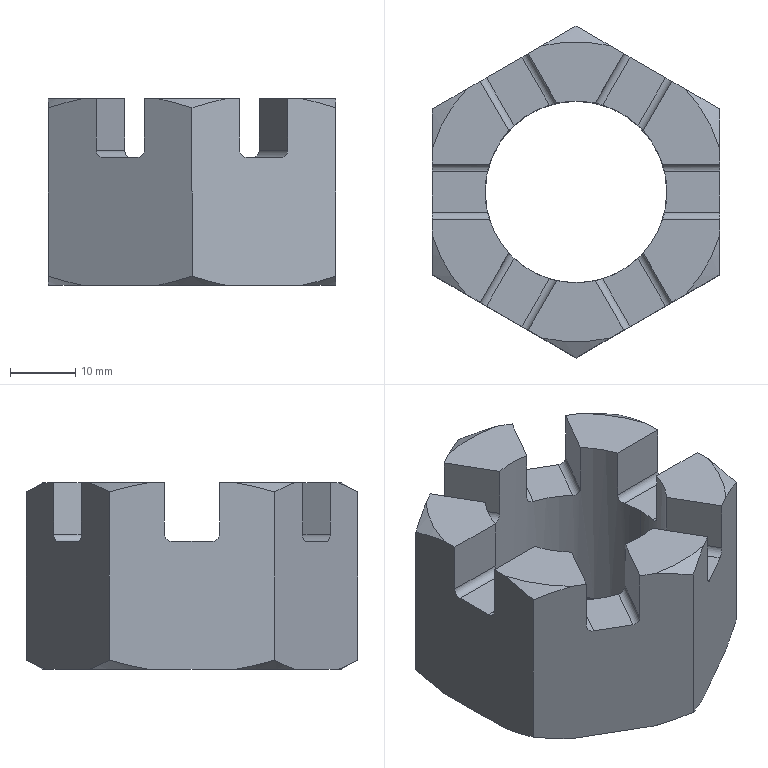Part | SolidWorks | features Cut 3, Chamfer 1, CirPattern 1, Extrusion 1 | 1 solid | 59 faces | box 44.037 x 50.85 x 28.6 mm | volume 26766 mm3 | plane 31 | cone 14 | cylinder 14 | commonest cylinder face diameters 2.25 x12 27.835 x2